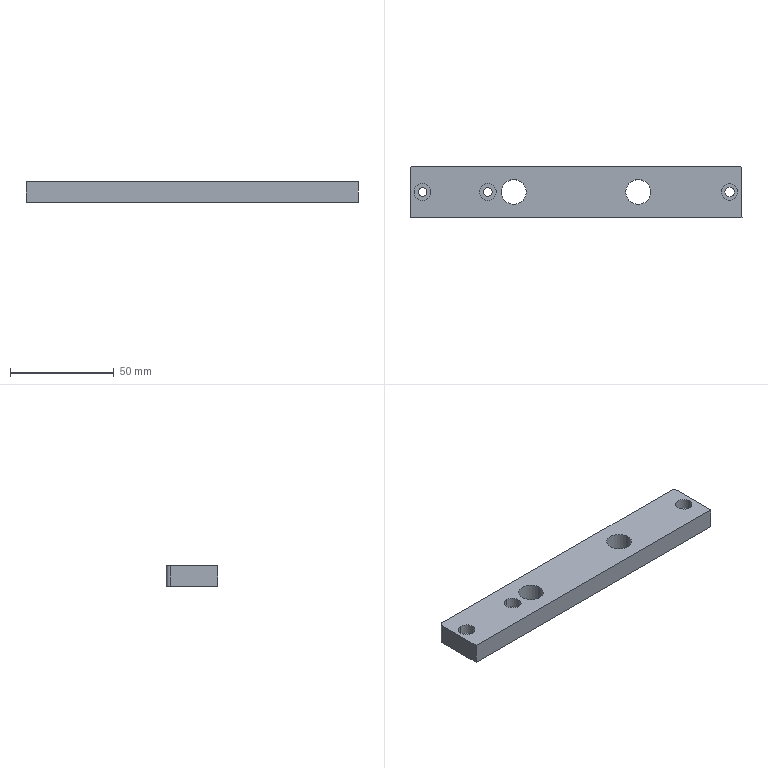Part | SolidWorks | features BaseBody 1, HoleWzd 1, MoveFace 1 | 1 solid | 31 faces | box 160 x 25 x 10 mm | volume 36749 mm3 | cylinder 22 | plane 9 | commonest cylinder face diameters 8 x8 4.2 x6 12 x4 4 x2 4.5 x2
STEP:
#1=CARTESIAN_POINT('',(-663.13,725.797,403.384));
#2=VERTEX_POINT('',#1);
#3=CARTESIAN_POINT('',(-655.13,725.797,403.384));
#4=VERTEX_POINT('',#3);
#5=CARTESIAN_POINT('',(-659.13,725.797,403.384));
#6=DIRECTION('',(0.,0.,1.));
#7=DIRECTION('',(1.,0.,0.));
#8=AXIS2_PLACEMENT_3D('',#5,#6,#7);
#9=CIRCLE('',#8,4.);
#10=EDGE_CURVE('',#2,#4,#9,.T.);
#11=ORIENTED_EDGE('',*,*,#10,.F.);
#12=CARTESIAN_POINT('',(-663.13,725.797,408.384));
#13=VERTEX_POINT('',#12);
#14=CARTESIAN_POINT('',(-663.13,725.797,408.384));
#15=DIRECTION('',(0.,0.,1.));
#16=VECTOR('',#15,1000.);
#17=LINE('',#14,#16);
#18=EDGE_CURVE('',#2,#13,#17,.T.);
#19=ORIENTED_EDGE('',*,*,#18,.T.);
#20=CARTESIAN_POINT('',(-655.13,725.797,408.384));
#21=VERTEX_POINT('',#20);
#22=CARTESIAN_POINT('',(-659.13,725.797,408.384));
#23=DIRECTION('',(0.,0.,1.));
#24=DIRECTION('',(1.,0.,0.));
#25=AXIS2_PLACEMENT_3D('',#22,#23,#24);
#26=CIRCLE('',#25,4.);
#27=EDGE_CURVE('',#13,#21,#26,.T.);
#28=ORIENTED_EDGE('',*,*,#27,.T.);
#29=CARTESIAN_POINT('',(-655.13,725.797,408.384));
#30=DIRECTION('',(0.,0.,1.));
#31=VECTOR('',#30,1000.);
#32=LINE('',#29,#31);
#33=EDGE_CURVE('',#4,#21,#32,.T.);
#34=ORIENTED_EDGE('',*,*,#33,.F.);
#35=EDGE_LOOP('',(#11,#19,#28,#34));
#36=FACE_OUTER_BOUND('',#35,.T.);
#37=CARTESIAN_POINT('',(-659.13,725.797,408.384));
#38=DIRECTION('',(0.,0.,1.));
#39=DIRECTION('',(1.,0.,0.));
#40=AXIS2_PLACEMENT_3D('',#37,#38,#39);
#41=CYLINDRICAL_SURFACE('',#40,4.);
#42=ADVANCED_FACE('',(#36),#41,.F.);
#43=CARTESIAN_POINT('',(-661.38,725.797,398.384));
#44=VERTEX_POINT('',#43);
#45=CARTESIAN_POINT('',(-656.88,725.797,398.384));
#46=VERTEX_POINT('',#45);
#47=CARTESIAN_POINT('',(-659.13,725.797,398.384));
#48=DIRECTION('',(0.,0.,1.));
#49=DIRECTION('',(1.,0.,0.));
#50=AXIS2_PLACEMENT_3D('',#47,#48,#49);
#51=CIRCLE('',#50,2.25);
#52=EDGE_CURVE('',#44,#46,#51,.T.);
#53=ORIENTED_EDGE('',*,*,#52,.F.);
#54=CARTESIAN_POINT('',(-661.38,725.797,403.384));
#55=VERTEX_POINT('',#54);
#56=CARTESIAN_POINT('',(-661.38,725.797,408.384));
#57=DIRECTION('',(0.,0.,1.));
#58=VECTOR('',#57,1000.);
#59=LINE('',#56,#58);
#60=EDGE_CURVE('',#44,#55,#59,.T.);
#61=ORIENTED_EDGE('',*,*,#60,.T.);
#62=CARTESIAN_POINT('',(-656.88,725.797,403.384));
#63=VERTEX_POINT('',#62);
#64=CARTESIAN_POINT('',(-659.13,725.797,403.384));
#65=DIRECTION('',(0.,0.,1.));
#66=DIRECTION('',(1.,0.,0.));
#67=AXIS2_PLACEMENT_3D('',#64,#65,#66);
#68=CIRCLE('',#67,2.25);
#69=EDGE_CURVE('',#55,#63,#68,.T.);
#70=ORIENTED_EDGE('',*,*,#69,.T.);
#71=CARTESIAN_POINT('',(-656.88,725.797,408.384));
#72=DIRECTION('',(0.,0.,1.));
#73=VECTOR('',#72,1000.);
#74=LINE('',#71,#73);
#75=EDGE_CURVE('',#46,#63,#74,.T.);
#76=ORIENTED_EDGE('',*,*,#75,.F.);
#77=EDGE_LOOP('',(#53,#61,#70,#76));
#78=FACE_OUTER_BOUND('',#77,.T.);
#79=CARTESIAN_POINT('',(-659.13,725.797,408.384));
#80=DIRECTION('',(0.,0.,1.));
#81=DIRECTION('',(1.,0.,0.));
#82=AXIS2_PLACEMENT_3D('',#79,#80,#81);
#83=CYLINDRICAL_SURFACE('',#82,2.25);
#84=ADVANCED_FACE('',(#78),#83,.F.);
#85=CARTESIAN_POINT('',(-807.13,723.697,398.384));
#86=VERTEX_POINT('',#85);
#87=CARTESIAN_POINT('',(-809.23,725.797,398.384));
#88=VERTEX_POINT('',#87);
#89=CARTESIAN_POINT('',(-807.13,725.797,398.384));
#90=DIRECTION('',(0.,0.,-1.));
#91=DIRECTION('',(-1.,-0.000001544,0.));
#92=AXIS2_PLACEMENT_3D('',#89,#90,#91);
#93=CIRCLE('',#92,2.1);
#94=EDGE_CURVE('',#86,#88,#93,.T.);
#95=ORIENTED_EDGE('',*,*,#94,.T.);
#96=CARTESIAN_POINT('',(-809.23,725.797,403.384));
#97=VERTEX_POINT('',#96);
#98=CARTESIAN_POINT('',(-809.23,725.797,408.384));
#99=DIRECTION('',(0.,0.,1.));
#100=VECTOR('',#99,1000.);
#101=LINE('',#98,#100);
#102=EDGE_CURVE('',#88,#97,#101,.T.);
#103=ORIENTED_EDGE('',*,*,#102,.T.);
#104=CARTESIAN_POINT('',(-807.13,723.697,403.384));
#105=VERTEX_POINT('',#104);
#106=CARTESIAN_POINT('',(-807.13,725.797,403.384));
#107=DIRECTION('',(0.,0.,1.));
#108=DIRECTION('',(-1.,-0.000001544,0.));
#109=AXIS2_PLACEMENT_3D('',#106,#107,#108);
#110=CIRCLE('',#109,2.1);
#111=EDGE_CURVE('',#97,#105,#110,.T.);
#112=ORIENTED_EDGE('',*,*,#111,.T.);
#113=CARTESIAN_POINT('',(-807.13,723.697,403.384));
#114=DIRECTION('',(0.,0.,-1.));
#115=VECTOR('',#114,1000.);
#116=LINE('',#113,#115);
#117=EDGE_CURVE('',#105,#86,#116,.T.);
#118=ORIENTED_EDGE('',*,*,#117,.T.);
#119=EDGE_LOOP('',(#95,#103,#112,#118));
#120=FACE_OUTER_BOUND('',#119,.T.);
#121=CARTESIAN_POINT('',(-807.13,725.797,408.384));
#122=DIRECTION('',(0.,0.,1.));
#123=DIRECTION('',(-1.,-0.000001544,0.));
#124=AXIS2_PLACEMENT_3D('',#121,#122,#123);
#125=CYLINDRICAL_SURFACE('',#124,2.1);
#126=ADVANCED_FACE('',(#120),#125,.F.);
#127=CARTESIAN_POINT('',(-807.13,721.797,403.384));
#128=VERTEX_POINT('',#127);
#129=CARTESIAN_POINT('',(-811.13,725.797,403.384));
#130=VERTEX_POINT('',#129);
#131=CARTESIAN_POINT('',(-807.13,725.797,403.384));
#132=DIRECTION('',(0.,0.,-1.));
#133=DIRECTION('',(-1.,-0.000001544,0.));
#134=AXIS2_PLACEMENT_3D('',#131,#132,#133);
#135=CIRCLE('',#134,4.);
#136=EDGE_CURVE('',#128,#130,#135,.T.);
#137=ORIENTED_EDGE('',*,*,#136,.T.);
#138=CARTESIAN_POINT('',(-811.13,725.797,408.384));
#139=VERTEX_POINT('',#138);
#140=CARTESIAN_POINT('',(-811.13,725.797,408.384));
#141=DIRECTION('',(0.,0.,1.));
#142=VECTOR('',#141,1000.);
#143=LINE('',#140,#142);
#144=EDGE_CURVE('',#130,#139,#143,.T.);
#145=ORIENTED_EDGE('',*,*,#144,.T.);
#146=CARTESIAN_POINT('',(-807.13,721.797,408.384));
#147=VERTEX_POINT('',#146);
#148=CARTESIAN_POINT('',(-807.13,725.797,408.384));
#149=DIRECTION('',(0.,0.,1.));
#150=DIRECTION('',(-1.,-0.000001544,0.));
#151=AXIS2_PLACEMENT_3D('',#148,#149,#150);
#152=CIRCLE('',#151,4.);
#153=EDGE_CURVE('',#139,#147,#152,.T.);
#154=ORIENTED_EDGE('',*,*,#153,.T.);
#155=CARTESIAN_POINT('',(-807.13,721.797,408.384));
#156=DIRECTION('',(0.,0.,-1.));
#157=VECTOR('',#156,1000.);
#158=LINE('',#155,#157);
#159=EDGE_CURVE('',#147,#128,#158,.T.);
#160=ORIENTED_EDGE('',*,*,#159,.T.);
#161=EDGE_LOOP('',(#137,#145,#154,#160));
#162=FACE_OUTER_BOUND('',#161,.T.);
#163=CARTESIAN_POINT('',(-807.13,725.797,408.384));
#164=DIRECTION('',(0.,0.,1.));
#165=DIRECTION('',(-1.,-0.000001544,0.));
#166=AXIS2_PLACEMENT_3D('',#163,#164,#165);
#167=CYLINDRICAL_SURFACE('',#166,4.);
#168=ADVANCED_FACE('',(#162),#167,.F.);
#169=CARTESIAN_POINT('',(-775.626,723.697,398.384));
#170=VERTEX_POINT('',#169);
#171=CARTESIAN_POINT('',(-777.726,725.797,398.384));
#172=VERTEX_POINT('',#171);
#173=CARTESIAN_POINT('',(-775.626,725.797,398.384));
#174=DIRECTION('',(0.,0.,-1.));
#175=DIRECTION('',(-1.,-0.000001544,0.));
#176=AXIS2_PLACEMENT_3D('',#173,#174,#175);
#177=CIRCLE('',#176,2.1);
#178=EDGE_CURVE('',#170,#172,#177,.T.);
#179=ORIENTED_EDGE('',*,*,#178,.T.);
#180=CARTESIAN_POINT('',(-777.726,725.797,403.384));
#181=VERTEX_POINT('',#180);
#182=CARTESIAN_POINT('',(-777.726,725.797,408.384));
#183=DIRECTION('',(0.,0.,1.));
#184=VECTOR('',#183,1000.);
#185=LINE('',#182,#184);
#186=EDGE_CURVE('',#172,#181,#185,.T.);
#187=ORIENTED_EDGE('',*,*,#186,.T.);
#188=CARTESIAN_POINT('',(-775.626,723.697,403.384));
#189=VERTEX_POINT('',#188);
#190=CARTESIAN_POINT('',(-775.626,725.797,403.384));
#191=DIRECTION('',(0.,0.,1.));
#192=DIRECTION('',(-1.,-0.000001544,0.));
#193=AXIS2_PLACEMENT_3D('',#190,#191,#192);
#194=CIRCLE('',#193,2.1);
#195=EDGE_CURVE('',#181,#189,#194,.T.);
#196=ORIENTED_EDGE('',*,*,#195,.T.);
#197=CARTESIAN_POINT('',(-775.626,723.697,403.384));
#198=DIRECTION('',(0.,0.,-1.));
#199=VECTOR('',#198,1000.);
#200=LINE('',#197,#199);
#201=EDGE_CURVE('',#189,#170,#200,.T.);
#202=ORIENTED_EDGE('',*,*,#201,.T.);
#203=EDGE_LOOP('',(#179,#187,#196,#202));
#204=FACE_OUTER_BOUND('',#203,.T.);
#205=CARTESIAN_POINT('',(-775.626,725.797,408.384));
#206=DIRECTION('',(0.,0.,1.));
#207=DIRECTION('',(-1.,-0.000001544,0.));
#208=AXIS2_PLACEMENT_3D('',#205,#206,#207);
#209=CYLINDRICAL_SURFACE('',#208,2.1);
#210=ADVANCED_FACE('',(#204),#209,.F.);
#211=CARTESIAN_POINT('',(-775.626,721.797,403.384));
#212=VERTEX_POINT('',#211);
#213=CARTESIAN_POINT('',(-779.626,725.797,403.384));
#214=VERTEX_POINT('',#213);
#215=CARTESIAN_POINT('',(-775.626,725.797,403.384));
#216=DIRECTION('',(0.,0.,-1.));
#217=DIRECTION('',(-1.,-0.000001544,0.));
#218=AXIS2_PLACEMENT_3D('',#215,#216,#217);
#219=CIRCLE('',#218,4.);
#220=EDGE_CURVE('',#212,#214,#219,.T.);
#221=ORIENTED_EDGE('',*,*,#220,.T.);
#222=CARTESIAN_POINT('',(-779.626,725.797,408.384));
#223=VERTEX_POINT('',#222);
#224=CARTESIAN_POINT('',(-779.626,725.797,408.384));
#225=DIRECTION('',(0.,0.,1.));
#226=VECTOR('',#225,1000.);
#227=LINE('',#224,#226);
#228=EDGE_CURVE('',#214,#223,#227,.T.);
#229=ORIENTED_EDGE('',*,*,#228,.T.);
#230=CARTESIAN_POINT('',(-775.626,721.797,408.384));
#231=VERTEX_POINT('',#230);
#232=CARTESIAN_POINT('',(-775.626,725.797,408.384));
#233=DIRECTION('',(0.,0.,1.));
#234=DIRECTION('',(-1.,-0.000001544,0.));
#235=AXIS2_PLACEMENT_3D('',#232,#233,#234);
#236=CIRCLE('',#235,4.);
#237=EDGE_CURVE('',#223,#231,#236,.T.);
#238=ORIENTED_EDGE('',*,*,#237,.T.);
#239=CARTESIAN_POINT('',(-775.626,721.797,408.384));
#240=DIRECTION('',(0.,0.,-1.));
#241=VECTOR('',#240,1000.);
#242=LINE('',#239,#241);
#243=EDGE_CURVE('',#231,#212,#242,.T.);
#244=ORIENTED_EDGE('',*,*,#243,.T.);
#245=EDGE_LOOP('',(#221,#229,#238,#244));
#246=FACE_OUTER_BOUND('',#245,.T.);
#247=CARTESIAN_POINT('',(-775.626,725.797,408.384));
#248=DIRECTION('',(0.,0.,1.));
#249=DIRECTION('',(-1.,-0.000001544,0.));
#250=AXIS2_PLACEMENT_3D('',#247,#248,#249);
#251=CYLINDRICAL_SURFACE('',#250,4.);
#252=ADVANCED_FACE('',(#246),#251,.F.);
#253=CARTESIAN_POINT('',(-813.13,713.297,408.384));
#254=VERTEX_POINT('',#253);
#255=CARTESIAN_POINT('',(-813.13,713.297,398.384));
#256=VERTEX_POINT('',#255);
#257=CARTESIAN_POINT('',(-813.13,713.297,408.384));
#258=DIRECTION('',(0.,0.,-1.));
#259=VECTOR('',#258,1000.);
#260=LINE('',#257,#259);
#261=EDGE_CURVE('',#254,#256,#260,.T.);
#262=ORIENTED_EDGE('',*,*,#261,.F.);
#263=CARTESIAN_POINT('',(-813.13,736.297,408.384));
#264=VERTEX_POINT('',#263);
#265=CARTESIAN_POINT('',(-813.13,736.297,408.384));
#266=DIRECTION('',(0.000001544,-1.,0.));
#267=VECTOR('',#266,1000.);
#268=LINE('',#265,#267);
#269=EDGE_CURVE('',#264,#254,#268,.T.);
#270=ORIENTED_EDGE('',*,*,#269,.F.);
#271=CARTESIAN_POINT('',(-813.13,736.297,398.384));
#272=VERTEX_POINT('',#271);
#273=CARTESIAN_POINT('',(-813.13,736.297,408.384));
#274=DIRECTION('',(0.,0.,-1.));
#275=VECTOR('',#274,1000.);
#276=LINE('',#273,#275);
#277=EDGE_CURVE('',#264,#272,#276,.T.);
#278=ORIENTED_EDGE('',*,*,#277,.T.);
#279=CARTESIAN_POINT('',(-813.13,713.297,398.384));
#280=DIRECTION('',(-0.000001544,1.,0.));
#281=VECTOR('',#280,1000.);
#282=LINE('',#279,#281);
#283=EDGE_CURVE('',#256,#272,#282,.T.);
#284=ORIENTED_EDGE('',*,*,#283,.F.);
#285=EDGE_LOOP('',(#262,#270,#278,#284));
#286=FACE_OUTER_BOUND('',#285,.T.);
#287=CARTESIAN_POINT('',(-813.129,0.00009293,-0.25));
#288=DIRECTION('',(-1.,-0.000001544,0.));
#289=DIRECTION('',(-0.000001544,1.,0.));
#290=AXIS2_PLACEMENT_3D('',#287,#288,#289);
#291=PLANE('',#290);
#292=ADVANCED_FACE('',(#286),#291,.T.);
#293=CARTESIAN_POINT('',(-659.13,725.797,398.384));
#294=DIRECTION('',(0.,0.,1.));
#295=DIRECTION('',(1.,0.,0.));
#296=AXIS2_PLACEMENT_3D('',#293,#294,#295);
#297=CIRCLE('',#296,2.25);
#298=EDGE_CURVE('',#46,#44,#297,.T.);
#299=ORIENTED_EDGE('',*,*,#298,.T.);
#300=ORIENTED_EDGE('',*,*,#52,.T.);
#301=EDGE_LOOP('',(#299,#300));
#302=FACE_BOUND('',#301,.T.);
#303=CARTESIAN_POINT('',(-653.13,736.297,398.384));
#304=VERTEX_POINT('',#303);
#305=CARTESIAN_POINT('',(-655.13,738.297,398.384));
#306=VERTEX_POINT('',#305);
#307=CARTESIAN_POINT('',(-655.13,736.297,398.384));
#308=DIRECTION('',(0.,0.,1.));
#309=DIRECTION('',(1.,0.000001544,0.));
#310=AXIS2_PLACEMENT_3D('',#307,#308,#309);
#311=CIRCLE('',#310,2.);
#312=EDGE_CURVE('',#304,#306,#311,.T.);
#313=ORIENTED_EDGE('',*,*,#312,.F.);
#314=CARTESIAN_POINT('',(-653.13,713.297,398.384));
#315=VERTEX_POINT('',#314);
#316=CARTESIAN_POINT('',(-653.13,713.297,398.384));
#317=DIRECTION('',(-0.000001544,1.,0.));
#318=VECTOR('',#317,1000.);
#319=LINE('',#316,#318);
#320=EDGE_CURVE('',#315,#304,#319,.T.);
#321=ORIENTED_EDGE('',*,*,#320,.F.);
#322=CARTESIAN_POINT('',(-813.13,713.297,398.384));
#323=DIRECTION('',(1.,0.000001544,0.));
#324=VECTOR('',#323,1000.);
#325=LINE('',#322,#324);
#326=EDGE_CURVE('',#256,#315,#325,.T.);
#327=ORIENTED_EDGE('',*,*,#326,.F.);
#328=ORIENTED_EDGE('',*,*,#283,.T.);
#329=CARTESIAN_POINT('',(-811.13,738.297,398.384));
#330=VERTEX_POINT('',#329);
#331=CARTESIAN_POINT('',(-811.13,736.297,398.384));
#332=DIRECTION('',(0.,0.,1.));
#333=DIRECTION('',(-0.000001544,1.,0.));
#334=AXIS2_PLACEMENT_3D('',#331,#332,#333);
#335=CIRCLE('',#334,2.);
#336=EDGE_CURVE('',#330,#272,#335,.T.);
#337=ORIENTED_EDGE('',*,*,#336,.F.);
#338=CARTESIAN_POINT('',(-655.13,738.297,398.384));
#339=DIRECTION('',(-1.,-0.000001544,0.));
#340=VECTOR('',#339,1000.);
#341=LINE('',#338,#340);
#342=EDGE_CURVE('',#306,#330,#341,.T.);
#343=ORIENTED_EDGE('',*,*,#342,.F.);
#344=EDGE_LOOP('',(#313,#321,#327,#328,#337,#343));
#345=FACE_OUTER_BOUND('',#344,.T.);
#346=ORIENTED_EDGE('',*,*,#178,.F.);
#347=CARTESIAN_POINT('',(-775.626,727.897,398.384));
#348=VERTEX_POINT('',#347);
#349=CARTESIAN_POINT('',(-775.626,725.797,398.384));
#350=DIRECTION('',(0.,0.,-1.));
#351=DIRECTION('',(-0.000001544,1.,0.));
#352=AXIS2_PLACEMENT_3D('',#349,#350,#351);
#353=CIRCLE('',#352,2.1);
#354=EDGE_CURVE('',#348,#170,#353,.T.);
#355=ORIENTED_EDGE('',*,*,#354,.F.);
#356=CARTESIAN_POINT('',(-775.626,725.797,398.384));
#357=DIRECTION('',(0.,0.,-1.));
#358=DIRECTION('',(-1.,-0.000001544,0.));
#359=AXIS2_PLACEMENT_3D('',#356,#357,#358);
#360=CIRCLE('',#359,2.1);
#361=EDGE_CURVE('',#172,#348,#360,.T.);
#362=ORIENTED_EDGE('',*,*,#361,.F.);
#363=EDGE_LOOP('',(#346,#355,#362));
#364=FACE_BOUND('',#363,.T.);
#365=ORIENTED_EDGE('',*,*,#94,.F.);
#366=CARTESIAN_POINT('',(-807.13,727.897,398.384));
#367=VERTEX_POINT('',#366);
#368=CARTESIAN_POINT('',(-807.13,725.797,398.384));
#369=DIRECTION('',(0.,0.,-1.));
#370=DIRECTION('',(-0.000001544,1.,0.));
#371=AXIS2_PLACEMENT_3D('',#368,#369,#370);
#372=CIRCLE('',#371,2.1);
#373=EDGE_CURVE('',#367,#86,#372,.T.);
#374=ORIENTED_EDGE('',*,*,#373,.F.);
#375=CARTESIAN_POINT('',(-807.13,725.797,398.384));
#376=DIRECTION('',(0.,0.,-1.));
#377=DIRECTION('',(-1.,-0.000001544,0.));
#378=AXIS2_PLACEMENT_3D('',#375,#376,#377);
#379=CIRCLE('',#378,2.1);
#380=EDGE_CURVE('',#88,#367,#379,.T.);
#381=ORIENTED_EDGE('',*,*,#380,.F.);
#382=EDGE_LOOP('',(#365,#374,#381));
#383=FACE_BOUND('',#382,.T.);
#384=CARTESIAN_POINT('',(-769.13,725.797,398.384));
#385=VERTEX_POINT('',#384);
#386=CARTESIAN_POINT('',(-757.13,725.797,398.384));
#387=VERTEX_POINT('',#386);
#388=CARTESIAN_POINT('',(-763.13,725.797,398.384));
#389=DIRECTION('',(0.,0.,-1.));
#390=DIRECTION('',(-1.,-0.000001544,0.));
#391=AXIS2_PLACEMENT_3D('',#388,#389,#390);
#392=CIRCLE('',#391,6.);
#393=EDGE_CURVE('',#385,#387,#392,.T.);
#394=ORIENTED_EDGE('',*,*,#393,.F.);
#395=CARTESIAN_POINT('',(-763.13,725.797,398.384));
#396=DIRECTION('',(0.,0.,-1.));
#397=DIRECTION('',(1.,0.000001544,0.));
#398=AXIS2_PLACEMENT_3D('',#395,#396,#397);
#399=CIRCLE('',#398,6.);
#400=EDGE_CURVE('',#387,#385,#399,.T.);
#401=ORIENTED_EDGE('',*,*,#400,.F.);
#402=EDGE_LOOP('',(#394,#401));
#403=FACE_BOUND('',#402,.T.);
#404=CARTESIAN_POINT('',(-709.13,725.797,398.384));
#405=VERTEX_POINT('',#404);
#406=CARTESIAN_POINT('',(-697.13,725.797,398.384));
#407=VERTEX_POINT('',#406);
#408=CARTESIAN_POINT('',(-703.13,725.797,398.384));
#409=DIRECTION('',(0.,0.,-1.));
#410=DIRECTION('',(-1.,-0.000001544,0.));
#411=AXIS2_PLACEMENT_3D('',#408,#409,#410);
#412=CIRCLE('',#411,6.);
#413=EDGE_CURVE('',#405,#407,#412,.T.);
#414=ORIENTED_EDGE('',*,*,#413,.F.);
#415=CARTESIAN_POINT('',(-703.13,725.797,398.384));
#416=DIRECTION('',(0.,0.,-1.));
#417=DIRECTION('',(1.,0.000001544,0.));
#418=AXIS2_PLACEMENT_3D('',#415,#416,#417);
#419=CIRCLE('',#418,6.);
#420=EDGE_CURVE('',#407,#405,#419,.T.);
#421=ORIENTED_EDGE('',*,*,#420,.F.);
#422=EDGE_LOOP('',(#414,#421));
#423=FACE_BOUND('',#422,.T.);
#424=CARTESIAN_POINT('',(-813.13,738.297,398.384));
#425=DIRECTION('',(0.,0.,-1.));
#426=DIRECTION('',(-0.000001544,1.,0.));
#427=AXIS2_PLACEMENT_3D('',#424,#425,#426);
#428=PLANE('',#427);
#429=ADVANCED_FACE('',(#302,#345,#364,#383,#403,#423),#428,.T.);
#430=CARTESIAN_POINT('',(-655.13,738.297,408.384));
#431=VERTEX_POINT('',#430);
#432=CARTESIAN_POINT('',(-655.13,738.297,408.384));
#433=DIRECTION('',(0.,0.,-1.));
#434=VECTOR('',#433,1000.);
#435=LINE('',#432,#434);
#436=EDGE_CURVE('',#431,#306,#435,.T.);
#437=ORIENTED_EDGE('',*,*,#436,.T.);
#438=ORIENTED_EDGE('',*,*,#342,.T.);
#439=CARTESIAN_POINT('',(-811.13,738.297,408.384));
#440=VERTEX_POINT('',#439);
#441=CARTESIAN_POINT('',(-811.13,738.297,398.384));
#442=DIRECTION('',(0.,0.,1.));
#443=VECTOR('',#442,1000.);
#444=LINE('',#441,#443);
#445=EDGE_CURVE('',#330,#440,#444,.T.);
#446=ORIENTED_EDGE('',*,*,#445,.T.);
#447=CARTESIAN_POINT('',(-811.13,738.297,408.384));
#448=DIRECTION('',(1.,0.000001544,0.));
#449=VECTOR('',#448,1000.);
#450=LINE('',#447,#449);
#451=EDGE_CURVE('',#440,#431,#450,.T.);
#452=ORIENTED_EDGE('',*,*,#451,.T.);
#453=EDGE_LOOP('',(#437,#438,#446,#452));
#454=FACE_OUTER_BOUND('',#453,.T.);
#455=CARTESIAN_POINT('',(-813.13,738.297,408.384));
#456=DIRECTION('',(-0.000001544,1.,0.));
#457=DIRECTION('',(0.,0.,1.));
#458=AXIS2_PLACEMENT_3D('',#455,#456,#457);
#459=PLANE('',#458);
#460=ADVANCED_FACE('',(#454),#459,.T.);
#461=CARTESIAN_POINT('',(-659.13,725.797,408.384));
#462=DIRECTION('',(0.,0.,1.));
#463=DIRECTION('',(1.,0.,0.));
#464=AXIS2_PLACEMENT_3D('',#461,#462,#463);
#465=CIRCLE('',#464,4.);
#466=EDGE_CURVE('',#21,#13,#465,.T.);
#467=ORIENTED_EDGE('',*,*,#466,.F.);
#468=ORIENTED_EDGE('',*,*,#27,.F.);
#469=EDGE_LOOP('',(#467,#468));
#470=FACE_BOUND('',#469,.T.);
#471=CARTESIAN_POINT('',(-653.13,713.297,408.384));
#472=VERTEX_POINT('',#471);
#473=CARTESIAN_POINT('',(-813.13,713.297,408.384));
#474=DIRECTION('',(1.,0.000001544,0.));
#475=VECTOR('',#474,1000.);
#476=LINE('',#473,#475);
#477=EDGE_CURVE('',#254,#472,#476,.T.);
#478=ORIENTED_EDGE('',*,*,#477,.T.);
#479=CARTESIAN_POINT('',(-653.13,736.297,408.384));
#480=VERTEX_POINT('',#479);
#481=CARTESIAN_POINT('',(-653.13,736.297,408.384));
#482=DIRECTION('',(0.000001544,-1.,0.));
#483=VECTOR('',#482,1000.);
#484=LINE('',#481,#483);
#485=EDGE_CURVE('',#480,#472,#484,.T.);
#486=ORIENTED_EDGE('',*,*,#485,.F.);
#487=CARTESIAN_POINT('',(-655.13,736.297,408.384));
#488=DIRECTION('',(0.,0.,-1.));
#489=DIRECTION('',(-0.000001544,1.,0.));
#490=AXIS2_PLACEMENT_3D('',#487,#488,#489);
#491=CIRCLE('',#490,2.);
#492=EDGE_CURVE('',#431,#480,#491,.T.);
#493=ORIENTED_EDGE('',*,*,#492,.F.);
#494=ORIENTED_EDGE('',*,*,#451,.F.);
#495=CARTESIAN_POINT('',(-811.13,736.297,408.384));
#496=DIRECTION('',(0.,0.,-1.));
#497=DIRECTION('',(-1.,-0.000001544,0.));
#498=AXIS2_PLACEMENT_3D('',#495,#496,#497);
#499=CIRCLE('',#498,2.);
#500=EDGE_CURVE('',#264,#440,#499,.T.);
#501=ORIENTED_EDGE('',*,*,#500,.F.);
#502=ORIENTED_EDGE('',*,*,#269,.T.);
#503=EDGE_LOOP('',(#478,#486,#493,#494,#501,#502));
#504=FACE_OUTER_BOUND('',#503,.T.);
#505=CARTESIAN_POINT('',(-775.626,729.797,408.384));
#506=VERTEX_POINT('',#505);
#507=CARTESIAN_POINT('',(-775.626,725.797,408.384));
#508=DIRECTION('',(0.,0.,1.));
#509=DIRECTION('',(-1.,-0.000001544,0.));
#510=AXIS2_PLACEMENT_3D('',#507,#508,#509);
#511=CIRCLE('',#510,4.);
#512=EDGE_CURVE('',#506,#223,#511,.T.);
#513=ORIENTED_EDGE('',*,*,#512,.F.);
#514=CARTESIAN_POINT('',(-775.626,725.797,408.384));
#515=DIRECTION('',(0.,0.,1.));
#516=DIRECTION('',(0.000001544,-1.,0.));
#517=AXIS2_PLACEMENT_3D('',#514,#515,#516);
#518=CIRCLE('',#517,4.);
#519=EDGE_CURVE('',#231,#506,#518,.T.);
#520=ORIENTED_EDGE('',*,*,#519,.F.);
#521=ORIENTED_EDGE('',*,*,#237,.F.);
#522=EDGE_LOOP('',(#513,#520,#521));
#523=FACE_BOUND('',#522,.T.);
#524=CARTESIAN_POINT('',(-807.13,729.797,408.384));
#525=VERTEX_POINT('',#524);
#526=CARTESIAN_POINT('',(-807.13,725.797,408.384));
#527=DIRECTION('',(0.,0.,1.));
#528=DIRECTION('',(-1.,-0.000001544,0.));
#529=AXIS2_PLACEMENT_3D('',#526,#527,#528);
#530=CIRCLE('',#529,4.);
#531=EDGE_CURVE('',#525,#139,#530,.T.);
#532=ORIENTED_EDGE('',*,*,#531,.F.);
#533=CARTESIAN_POINT('',(-807.13,725.797,408.384));
#534=DIRECTION('',(0.,0.,1.));
#535=DIRECTION('',(0.000001544,-1.,0.));
#536=AXIS2_PLACEMENT_3D('',#533,#534,#535);
#537=CIRCLE('',#536,4.);
#538=EDGE_CURVE('',#147,#525,#537,.T.);
#539=ORIENTED_EDGE('',*,*,#538,.F.);
#540=ORIENTED_EDGE('',*,*,#153,.F.);
#541=EDGE_LOOP('',(#532,#539,#540));
#542=FACE_BOUND('',#541,.T.);
#543=CARTESIAN_POINT('',(-757.13,725.797,408.384));
#544=VERTEX_POINT('',#543);
#545=CARTESIAN_POINT('',(-769.13,725.797,408.384));
#546=VERTEX_POINT('',#545);
#547=CARTESIAN_POINT('',(-763.13,725.797,408.384));
#548=DIRECTION('',(0.,0.,1.));
#549=DIRECTION('',(1.,0.000001544,0.));
#550=AXIS2_PLACEMENT_3D('',#547,#548,#549);
#551=CIRCLE('',#550,6.);
#552=EDGE_CURVE('',#544,#546,#551,.T.);
#553=ORIENTED_EDGE('',*,*,#552,.F.);
#554=CARTESIAN_POINT('',(-763.13,725.797,408.384));
#555=DIRECTION('',(0.,0.,1.));
#556=DIRECTION('',(-1.,-0.000001544,0.));
#557=AXIS2_PLACEMENT_3D('',#554,#555,#556);
#558=CIRCLE('',#557,6.);
#559=EDGE_CURVE('',#546,#544,#558,.T.);
#560=ORIENTED_EDGE('',*,*,#559,.F.);
#561=EDGE_LOOP('',(#553,#560));
#562=FACE_BOUND('',#561,.T.);
#563=CARTESIAN_POINT('',(-697.13,725.797,408.384));
#564=VERTEX_POINT('',#563);
#565=CARTESIAN_POINT('',(-709.13,725.797,408.384));
#566=VERTEX_POINT('',#565);
#567=CARTESIAN_POINT('',(-703.13,725.797,408.384));
#568=DIRECTION('',(0.,0.,1.));
#569=DIRECTION('',(1.,0.000001544,0.));
#570=AXIS2_PLACEMENT_3D('',#567,#568,#569);
#571=CIRCLE('',#570,6.);
#572=EDGE_CURVE('',#564,#566,#571,.T.);
#573=ORIENTED_EDGE('',*,*,#572,.F.);
#574=CARTESIAN_POINT('',(-703.13,725.797,408.384));
#575=DIRECTION('',(0.,0.,1.));
#576=DIRECTION('',(-1.,-0.000001544,0.));
#577=AXIS2_PLACEMENT_3D('',#574,#575,#576);
#578=CIRCLE('',#577,6.);
#579=EDGE_CURVE('',#566,#564,#578,.T.);
#580=ORIENTED_EDGE('',*,*,#579,.F.);
#581=EDGE_LOOP('',(#573,#580));
#582=FACE_BOUND('',#581,.T.);
#583=CARTESIAN_POINT('',(-813.13,713.297,408.384));
#584=DIRECTION('',(0.,0.,1.));
#585=DIRECTION('',(0.000001544,-1.,0.));
#586=AXIS2_PLACEMENT_3D('',#583,#584,#585);
#587=PLANE('',#586);
#588=ADVANCED_FACE('',(#470,#504,#523,#542,#562,#582),#587,.T.);
#589=ORIENTED_EDGE('',*,*,#500,.T.);
#590=ORIENTED_EDGE('',*,*,#445,.F.);
#591=ORIENTED_EDGE('',*,*,#336,.T.);
#592=ORIENTED_EDGE('',*,*,#277,.F.);
#593=EDGE_LOOP('',(#589,#590,#591,#592));
#594=FACE_OUTER_BOUND('',#593,.T.);
#595=CARTESIAN_POINT('',(-811.13,736.297,421.42));
#596=DIRECTION('',(0.,0.,-1.));
#597=DIRECTION('',(1.,0.000001544,0.));
#598=AXIS2_PLACEMENT_3D('',#595,#596,#597);
#599=CYLINDRICAL_SURFACE('',#598,2.);
#600=ADVANCED_FACE('',(#594),#599,.T.);
#601=ORIENTED_EDGE('',*,*,#312,.T.);
#602=ORIENTED_EDGE('',*,*,#436,.F.);
#603=ORIENTED_EDGE('',*,*,#492,.T.);
#604=CARTESIAN_POINT('',(-653.13,736.297,398.384));
#605=DIRECTION('',(0.,0.,1.));
#606=VECTOR('',#605,1000.);
#607=LINE('',#604,#606);
#608=EDGE_CURVE('',#304,#480,#607,.T.);
#609=ORIENTED_EDGE('',*,*,#608,.F.);
#610=EDGE_LOOP('',(#601,#602,#603,#609));
#611=FACE_OUTER_BOUND('',#610,.T.);
#612=CARTESIAN_POINT('',(-655.13,736.297,385.348));
#613=DIRECTION('',(0.,0.,1.));
#614=DIRECTION('',(-1.,-0.000001544,0.));
#615=AXIS2_PLACEMENT_3D('',#612,#613,#614);
#616=CYLINDRICAL_SURFACE('',#615,2.);
#617=ADVANCED_FACE('',(#611),#616,.T.);
#618=CARTESIAN_POINT('',(-653.13,713.297,408.384));
#619=DIRECTION('',(0.,0.,-1.));
#620=VECTOR('',#619,1000.);
#621=LINE('',#618,#620);
#622=EDGE_CURVE('',#472,#315,#621,.T.);
#623=ORIENTED_EDGE('',*,*,#622,.T.);
#624=ORIENTED_EDGE('',*,*,#320,.T.);
#625=ORIENTED_EDGE('',*,*,#608,.T.);
#626=ORIENTED_EDGE('',*,*,#485,.T.);
#627=EDGE_LOOP('',(#623,#624,#625,#626));
#628=FACE_OUTER_BOUND('',#627,.T.);
#629=CARTESIAN_POINT('',(-653.129,0.00034,-0.25));
#630=DIRECTION('',(1.,0.000001544,0.));
#631=DIRECTION('',(0.000001544,-1.,0.));
#632=AXIS2_PLACEMENT_3D('',#629,#630,#631);
#633=PLANE('',#632);
#634=ADVANCED_FACE('',(#628),#633,.T.);
#635=ORIENTED_EDGE('',*,*,#622,.F.);
#636=ORIENTED_EDGE('',*,*,#477,.F.);
#637=ORIENTED_EDGE('',*,*,#261,.T.);
#638=ORIENTED_EDGE('',*,*,#326,.T.);
#639=EDGE_LOOP('',(#635,#636,#637,#638));
#640=FACE_OUTER_BOUND('',#639,.T.);
#641=CARTESIAN_POINT('',(-813.13,713.297,398.384));
#642=DIRECTION('',(0.000001544,-1.,0.));
#643=DIRECTION('',(0.,0.,-1.));
#644=AXIS2_PLACEMENT_3D('',#641,#642,#643);
#645=PLANE('',#644);
#646=ADVANCED_FACE('',(#640),#645,.T.);
#647=ORIENTED_EDGE('',*,*,#228,.F.);
#648=CARTESIAN_POINT('',(-775.626,729.797,403.384));
#649=VERTEX_POINT('',#648);
#650=CARTESIAN_POINT('',(-775.626,725.797,403.384));
#651=DIRECTION('',(0.,0.,-1.));
#652=DIRECTION('',(-1.,-0.000001544,0.));
#653=AXIS2_PLACEMENT_3D('',#650,#651,#652);
#654=CIRCLE('',#653,4.);
#655=EDGE_CURVE('',#214,#649,#654,.T.);
#656=ORIENTED_EDGE('',*,*,#655,.T.);
#657=CARTESIAN_POINT('',(-775.626,729.797,403.384));
#658=DIRECTION('',(0.,0.,1.));
#659=VECTOR('',#658,1000.);
#660=LINE('',#657,#659);
#661=EDGE_CURVE('',#649,#506,#660,.T.);
#662=ORIENTED_EDGE('',*,*,#661,.T.);
#663=ORIENTED_EDGE('',*,*,#512,.T.);
#664=EDGE_LOOP('',(#647,#656,#662,#663));
#665=FACE_OUTER_BOUND('',#664,.T.);
#666=CARTESIAN_POINT('',(-775.626,725.797,408.384));
#667=DIRECTION('',(0.,0.,1.));
#668=DIRECTION('',(-1.,-0.000001544,0.));
#669=AXIS2_PLACEMENT_3D('',#666,#667,#668);
#670=CYLINDRICAL_SURFACE('',#669,4.);
#671=ADVANCED_FACE('',(#665),#670,.F.);
#672=ORIENTED_EDGE('',*,*,#661,.F.);
#673=CARTESIAN_POINT('',(-775.626,725.797,403.384));
#674=DIRECTION('',(0.,0.,-1.));
#675=DIRECTION('',(1.,0.000001544,0.));
#676=AXIS2_PLACEMENT_3D('',#673,#674,#675);
#677=CIRCLE('',#676,4.);
#678=EDGE_CURVE('',#649,#212,#677,.T.);
#679=ORIENTED_EDGE('',*,*,#678,.T.);
#680=ORIENTED_EDGE('',*,*,#243,.F.);
#681=ORIENTED_EDGE('',*,*,#519,.T.);
#682=EDGE_LOOP('',(#672,#679,#680,#681));
#683=FACE_OUTER_BOUND('',#682,.T.);
#684=CARTESIAN_POINT('',(-775.626,725.797,408.384));
#685=DIRECTION('',(0.,0.,1.));
#686=DIRECTION('',(-1.,-0.000001544,0.));
#687=AXIS2_PLACEMENT_3D('',#684,#685,#686);
#688=CYLINDRICAL_SURFACE('',#687,4.);
#689=ADVANCED_FACE('',(#683),#688,.F.);
#690=ORIENTED_EDGE('',*,*,#220,.F.);
#691=ORIENTED_EDGE('',*,*,#678,.F.);
#692=ORIENTED_EDGE('',*,*,#655,.F.);
#693=EDGE_LOOP('',(#690,#691,#692));
#694=FACE_OUTER_BOUND('',#693,.T.);
#695=CARTESIAN_POINT('',(-775.626,727.897,403.384));
#696=VERTEX_POINT('',#695);
#697=CARTESIAN_POINT('',(-775.626,725.797,403.384));
#698=DIRECTION('',(0.,0.,1.));
#699=DIRECTION('',(-1.,-0.000001544,0.));
#700=AXIS2_PLACEMENT_3D('',#697,#698,#699);
#701=CIRCLE('',#700,2.1);
#702=EDGE_CURVE('',#696,#181,#701,.T.);
#703=ORIENTED_EDGE('',*,*,#702,.F.);
#704=CARTESIAN_POINT('',(-775.626,725.797,403.384));
#705=DIRECTION('',(0.,0.,1.));
#706=DIRECTION('',(0.000001544,-1.,0.));
#707=AXIS2_PLACEMENT_3D('',#704,#705,#706);
#708=CIRCLE('',#707,2.1);
#709=EDGE_CURVE('',#189,#696,#708,.T.);
#710=ORIENTED_EDGE('',*,*,#709,.F.);
#711=ORIENTED_EDGE('',*,*,#195,.F.);
#712=EDGE_LOOP('',(#703,#710,#711));
#713=FACE_BOUND('',#712,.T.);
#714=CARTESIAN_POINT('',(-813.129,0.00009293,403.384));
#715=DIRECTION('',(0.,0.,1.));
#716=DIRECTION('',(-0.000001544,1.,0.));
#717=AXIS2_PLACEMENT_3D('',#714,#715,#716);
#718=PLANE('',#717);
#719=ADVANCED_FACE('',(#694,#713),#718,.T.);
#720=ORIENTED_EDGE('',*,*,#186,.F.);
#721=ORIENTED_EDGE('',*,*,#361,.T.);
#722=CARTESIAN_POINT('',(-775.626,727.897,398.384));
#723=DIRECTION('',(0.,0.,1.));
#724=VECTOR('',#723,1000.);
#725=LINE('',#722,#724);
#726=EDGE_CURVE('',#348,#696,#725,.T.);
#727=ORIENTED_EDGE('',*,*,#726,.T.);
#728=ORIENTED_EDGE('',*,*,#702,.T.);
#729=EDGE_LOOP('',(#720,#721,#727,#728));
#730=FACE_OUTER_BOUND('',#729,.T.);
#731=CARTESIAN_POINT('',(-775.626,725.797,408.384));
#732=DIRECTION('',(0.,0.,1.));
#733=DIRECTION('',(-1.,-0.000001544,0.));
#734=AXIS2_PLACEMENT_3D('',#731,#732,#733);
#735=CYLINDRICAL_SURFACE('',#734,2.1);
#736=ADVANCED_FACE('',(#730),#735,.F.);
#737=ORIENTED_EDGE('',*,*,#354,.T.);
#738=ORIENTED_EDGE('',*,*,#201,.F.);
#739=ORIENTED_EDGE('',*,*,#709,.T.);
#740=ORIENTED_EDGE('',*,*,#726,.F.);
#741=EDGE_LOOP('',(#737,#738,#739,#740));
#742=FACE_OUTER_BOUND('',#741,.T.);
#743=CARTESIAN_POINT('',(-775.626,725.797,408.384));
#744=DIRECTION('',(0.,0.,1.));
#745=DIRECTION('',(-1.,-0.000001544,0.));
#746=AXIS2_PLACEMENT_3D('',#743,#744,#745);
#747=CYLINDRICAL_SURFACE('',#746,2.1);
#748=ADVANCED_FACE('',(#742),#747,.F.);
#749=ORIENTED_EDGE('',*,*,#144,.F.);
#750=CARTESIAN_POINT('',(-807.13,729.797,403.384));
#751=VERTEX_POINT('',#750);
#752=CARTESIAN_POINT('',(-807.13,725.797,403.384));
#753=DIRECTION('',(0.,0.,-1.));
#754=DIRECTION('',(-1.,-0.000001544,0.));
#755=AXIS2_PLACEMENT_3D('',#752,#753,#754);
#756=CIRCLE('',#755,4.);
#757=EDGE_CURVE('',#130,#751,#756,.T.);
#758=ORIENTED_EDGE('',*,*,#757,.T.);
#759=CARTESIAN_POINT('',(-807.13,729.797,403.384));
#760=DIRECTION('',(0.,0.,1.));
#761=VECTOR('',#760,1000.);
#762=LINE('',#759,#761);
#763=EDGE_CURVE('',#751,#525,#762,.T.);
#764=ORIENTED_EDGE('',*,*,#763,.T.);
#765=ORIENTED_EDGE('',*,*,#531,.T.);
#766=EDGE_LOOP('',(#749,#758,#764,#765));
#767=FACE_OUTER_BOUND('',#766,.T.);
#768=CARTESIAN_POINT('',(-807.13,725.797,408.384));
#769=DIRECTION('',(0.,0.,1.));
#770=DIRECTION('',(-1.,-0.000001544,0.));
#771=AXIS2_PLACEMENT_3D('',#768,#769,#770);
#772=CYLINDRICAL_SURFACE('',#771,4.);
#773=ADVANCED_FACE('',(#767),#772,.F.);
#774=ORIENTED_EDGE('',*,*,#763,.F.);
#775=CARTESIAN_POINT('',(-807.13,725.797,403.384));
#776=DIRECTION('',(0.,0.,-1.));
#777=DIRECTION('',(1.,0.000001544,0.));
#778=AXIS2_PLACEMENT_3D('',#775,#776,#777);
#779=CIRCLE('',#778,4.);
#780=EDGE_CURVE('',#751,#128,#779,.T.);
#781=ORIENTED_EDGE('',*,*,#780,.T.);
#782=ORIENTED_EDGE('',*,*,#159,.F.);
#783=ORIENTED_EDGE('',*,*,#538,.T.);
#784=EDGE_LOOP('',(#774,#781,#782,#783));
#785=FACE_OUTER_BOUND('',#784,.T.);
#786=CARTESIAN_POINT('',(-807.13,725.797,408.384));
#787=DIRECTION('',(0.,0.,1.));
#788=DIRECTION('',(-1.,-0.000001544,0.));
#789=AXIS2_PLACEMENT_3D('',#786,#787,#788);
#790=CYLINDRICAL_SURFACE('',#789,4.);
#791=ADVANCED_FACE('',(#785),#790,.F.);
#792=ORIENTED_EDGE('',*,*,#136,.F.);
#793=ORIENTED_EDGE('',*,*,#780,.F.);
#794=ORIENTED_EDGE('',*,*,#757,.F.);
#795=EDGE_LOOP('',(#792,#793,#794));
#796=FACE_OUTER_BOUND('',#795,.T.);
#797=CARTESIAN_POINT('',(-807.13,727.897,403.384));
#798=VERTEX_POINT('',#797);
#799=CARTESIAN_POINT('',(-807.13,725.797,403.384));
#800=DIRECTION('',(0.,0.,1.));
#801=DIRECTION('',(-1.,-0.000001544,0.));
#802=AXIS2_PLACEMENT_3D('',#799,#800,#801);
#803=CIRCLE('',#802,2.1);
#804=EDGE_CURVE('',#798,#97,#803,.T.);
#805=ORIENTED_EDGE('',*,*,#804,.F.);
#806=CARTESIAN_POINT('',(-807.13,725.797,403.384));
#807=DIRECTION('',(0.,0.,1.));
#808=DIRECTION('',(0.000001544,-1.,0.));
#809=AXIS2_PLACEMENT_3D('',#806,#807,#808);
#810=CIRCLE('',#809,2.1);
#811=EDGE_CURVE('',#105,#798,#810,.T.);
#812=ORIENTED_EDGE('',*,*,#811,.F.);
#813=ORIENTED_EDGE('',*,*,#111,.F.);
#814=EDGE_LOOP('',(#805,#812,#813));
#815=FACE_BOUND('',#814,.T.);
#816=CARTESIAN_POINT('',(-813.129,0.00009293,403.384));
#817=DIRECTION('',(0.,0.,1.));
#818=DIRECTION('',(-0.000001544,1.,0.));
#819=AXIS2_PLACEMENT_3D('',#816,#817,#818);
#820=PLANE('',#819);
#821=ADVANCED_FACE('',(#796,#815),#820,.T.);
#822=ORIENTED_EDGE('',*,*,#102,.F.);
#823=ORIENTED_EDGE('',*,*,#380,.T.);
#824=CARTESIAN_POINT('',(-807.13,727.897,398.384));
#825=DIRECTION('',(0.,0.,1.));
#826=VECTOR('',#825,1000.);
#827=LINE('',#824,#826);
#828=EDGE_CURVE('',#367,#798,#827,.T.);
#829=ORIENTED_EDGE('',*,*,#828,.T.);
#830=ORIENTED_EDGE('',*,*,#804,.T.);
#831=EDGE_LOOP('',(#822,#823,#829,#830));
#832=FACE_OUTER_BOUND('',#831,.T.);
#833=CARTESIAN_POINT('',(-807.13,725.797,408.384));
#834=DIRECTION('',(0.,0.,1.));
#835=DIRECTION('',(-1.,-0.000001544,0.));
#836=AXIS2_PLACEMENT_3D('',#833,#834,#835);
#837=CYLINDRICAL_SURFACE('',#836,2.1);
#838=ADVANCED_FACE('',(#832),#837,.F.);
#839=ORIENTED_EDGE('',*,*,#373,.T.);
#840=ORIENTED_EDGE('',*,*,#117,.F.);
#841=ORIENTED_EDGE('',*,*,#811,.T.);
#842=ORIENTED_EDGE('',*,*,#828,.F.);
#843=EDGE_LOOP('',(#839,#840,#841,#842));
#844=FACE_OUTER_BOUND('',#843,.T.);
#845=CARTESIAN_POINT('',(-807.13,725.797,408.384));
#846=DIRECTION('',(0.,0.,1.));
#847=DIRECTION('',(-1.,-0.000001544,0.));
#848=AXIS2_PLACEMENT_3D('',#845,#846,#847);
#849=CYLINDRICAL_SURFACE('',#848,2.1);
#850=ADVANCED_FACE('',(#844),#849,.F.);
#851=ORIENTED_EDGE('',*,*,#559,.T.);
#852=CARTESIAN_POINT('',(-757.13,725.797,408.384));
#853=DIRECTION('',(0.,0.,-1.));
#854=VECTOR('',#853,1000.);
#855=LINE('',#852,#854);
#856=EDGE_CURVE('',#544,#387,#855,.T.);
#857=ORIENTED_EDGE('',*,*,#856,.T.);
#858=ORIENTED_EDGE('',*,*,#400,.T.);
#859=CARTESIAN_POINT('',(-769.13,725.797,398.384));
#860=DIRECTION('',(0.,0.,1.));
#861=VECTOR('',#860,1000.);
#862=LINE('',#859,#861);
#863=EDGE_CURVE('',#385,#546,#862,.T.);
#864=ORIENTED_EDGE('',*,*,#863,.T.);
#865=EDGE_LOOP('',(#851,#857,#858,#864));
#866=FACE_OUTER_BOUND('',#865,.T.);
#867=CARTESIAN_POINT('',(-763.13,725.797,408.384));
#868=DIRECTION('',(0.,0.,1.));
#869=DIRECTION('',(-1.,-0.000001544,0.));
#870=AXIS2_PLACEMENT_3D('',#867,#868,#869);
#871=CYLINDRICAL_SURFACE('',#870,6.);
#872=ADVANCED_FACE('',(#866),#871,.F.);
#873=ORIENTED_EDGE('',*,*,#552,.T.);
#874=ORIENTED_EDGE('',*,*,#863,.F.);
#875=ORIENTED_EDGE('',*,*,#393,.T.);
#876=ORIENTED_EDGE('',*,*,#856,.F.);
#877=EDGE_LOOP('',(#873,#874,#875,#876));
#878=FACE_OUTER_BOUND('',#877,.T.);
#879=CARTESIAN_POINT('',(-763.13,725.797,408.384));
#880=DIRECTION('',(0.,0.,1.));
#881=DIRECTION('',(-1.,-0.000001544,0.));
#882=AXIS2_PLACEMENT_3D('',#879,#880,#881);
#883=CYLINDRICAL_SURFACE('',#882,6.);
#884=ADVANCED_FACE('',(#878),#883,.F.);
#885=ORIENTED_EDGE('',*,*,#579,.T.);
#886=CARTESIAN_POINT('',(-697.13,725.797,408.384));
#887=DIRECTION('',(0.,0.,-1.));
#888=VECTOR('',#887,1000.);
#889=LINE('',#886,#888);
#890=EDGE_CURVE('',#564,#407,#889,.T.);
#891=ORIENTED_EDGE('',*,*,#890,.T.);
#892=ORIENTED_EDGE('',*,*,#420,.T.);
#893=CARTESIAN_POINT('',(-709.13,725.797,398.384));
#894=DIRECTION('',(0.,0.,1.));
#895=VECTOR('',#894,1000.);
#896=LINE('',#893,#895);
#897=EDGE_CURVE('',#405,#566,#896,.T.);
#898=ORIENTED_EDGE('',*,*,#897,.T.);
#899=EDGE_LOOP('',(#885,#891,#892,#898));
#900=FACE_OUTER_BOUND('',#899,.T.);
#901=CARTESIAN_POINT('',(-703.13,725.797,408.384));
#902=DIRECTION('',(0.,0.,1.));
#903=DIRECTION('',(-1.,-0.000001544,0.));
#904=AXIS2_PLACEMENT_3D('',#901,#902,#903);
#905=CYLINDRICAL_SURFACE('',#904,6.);
#906=ADVANCED_FACE('',(#900),#905,.F.);
#907=ORIENTED_EDGE('',*,*,#572,.T.);
#908=ORIENTED_EDGE('',*,*,#897,.F.);
#909=ORIENTED_EDGE('',*,*,#413,.T.);
#910=ORIENTED_EDGE('',*,*,#890,.F.);
#911=EDGE_LOOP('',(#907,#908,#909,#910));
#912=FACE_OUTER_BOUND('',#911,.T.);
#913=CARTESIAN_POINT('',(-703.13,725.797,408.384));
#914=DIRECTION('',(0.,0.,1.));
#915=DIRECTION('',(-1.,-0.000001544,0.));
#916=AXIS2_PLACEMENT_3D('',#913,#914,#915);
#917=CYLINDRICAL_SURFACE('',#916,6.);
#918=ADVANCED_FACE('',(#912),#917,.F.);
#919=ORIENTED_EDGE('',*,*,#60,.F.);
#920=ORIENTED_EDGE('',*,*,#298,.F.);
#921=ORIENTED_EDGE('',*,*,#75,.T.);
#922=CARTESIAN_POINT('',(-659.13,725.797,403.384));
#923=DIRECTION('',(0.,0.,1.));
#924=DIRECTION('',(1.,0.,0.));
#925=AXIS2_PLACEMENT_3D('',#922,#923,#924);
#926=CIRCLE('',#925,2.25);
#927=EDGE_CURVE('',#63,#55,#926,.T.);
#928=ORIENTED_EDGE('',*,*,#927,.T.);
#929=EDGE_LOOP('',(#919,#920,#921,#928));
#930=FACE_OUTER_BOUND('',#929,.T.);
#931=CARTESIAN_POINT('',(-659.13,725.797,408.384));
#932=DIRECTION('',(0.,0.,1.));
#933=DIRECTION('',(1.,0.,0.));
#934=AXIS2_PLACEMENT_3D('',#931,#932,#933);
#935=CYLINDRICAL_SURFACE('',#934,2.25);
#936=ADVANCED_FACE('',(#930),#935,.F.);
#937=ORIENTED_EDGE('',*,*,#18,.F.);
#938=CARTESIAN_POINT('',(-659.13,725.797,403.384));
#939=DIRECTION('',(0.,0.,1.));
#940=DIRECTION('',(1.,0.,0.));
#941=AXIS2_PLACEMENT_3D('',#938,#939,#940);
#942=CIRCLE('',#941,4.);
#943=EDGE_CURVE('',#4,#2,#942,.T.);
#944=ORIENTED_EDGE('',*,*,#943,.F.);
#945=ORIENTED_EDGE('',*,*,#33,.T.);
#946=ORIENTED_EDGE('',*,*,#466,.T.);
#947=EDGE_LOOP('',(#937,#944,#945,#946));
#948=FACE_OUTER_BOUND('',#947,.T.);
#949=CARTESIAN_POINT('',(-659.13,725.797,408.384));
#950=DIRECTION('',(0.,0.,1.));
#951=DIRECTION('',(1.,0.,0.));
#952=AXIS2_PLACEMENT_3D('',#949,#950,#951);
#953=CYLINDRICAL_SURFACE('',#952,4.);
#954=ADVANCED_FACE('',(#948),#953,.F.);
#955=ORIENTED_EDGE('',*,*,#927,.F.);
#956=ORIENTED_EDGE('',*,*,#69,.F.);
#957=EDGE_LOOP('',(#955,#956));
#958=FACE_BOUND('',#957,.T.);
#959=ORIENTED_EDGE('',*,*,#943,.T.);
#960=ORIENTED_EDGE('',*,*,#10,.T.);
#961=EDGE_LOOP('',(#959,#960));
#962=FACE_OUTER_BOUND('',#961,.T.);
#963=CARTESIAN_POINT('',(-813.129,0.00009293,403.384));
#964=DIRECTION('',(0.,0.,1.));
#965=DIRECTION('',(-0.000001544,1.,0.));
#966=AXIS2_PLACEMENT_3D('',#963,#964,#965);
#967=PLANE('',#966);
#968=ADVANCED_FACE('',(#958,#962),#967,.T.);
#969=CLOSED_SHELL('',(#42,#84,#126,#168,#210,#252,#292,#429,#460,#588,#600,#617,#634,#646,#671,#689,#719,#736,#748,#773,#791,#821,#838,#850,#872,#884,#906,#918,#936,#954,#968));
#970=MANIFOLD_SOLID_BREP('',#969);
#971=CARTESIAN_POINT('',(0.,0.,0.));
#972=DIRECTION('',(0.,0.,1.));
#973=DIRECTION('',(1.,0.,0.));
#974=AXIS2_PLACEMENT_3D('',#971,#972,#973);
#975=(LENGTH_UNIT()NAMED_UNIT(*)SI_UNIT(.MILLI.,.METRE.));
#976=UNCERTAINTY_MEASURE_WITH_UNIT(LENGTH_MEASURE(0.00001),#975,'','');
#977=(NAMED_UNIT(*)PLANE_ANGLE_UNIT()SI_UNIT($,.RADIAN.));
#978=(NAMED_UNIT(*)SI_UNIT($,.STERADIAN.)SOLID_ANGLE_UNIT());
#979=(GEOMETRIC_REPRESENTATION_CONTEXT(3)GLOBAL_UNCERTAINTY_ASSIGNED_CONTEXT((#976))GLOBAL_UNIT_ASSIGNED_CONTEXT((#975,#977,#978))REPRESENTATION_CONTEXT('',''));
#980=ADVANCED_BREP_SHAPE_REPRESENTATION('',(#970,#974),#979);